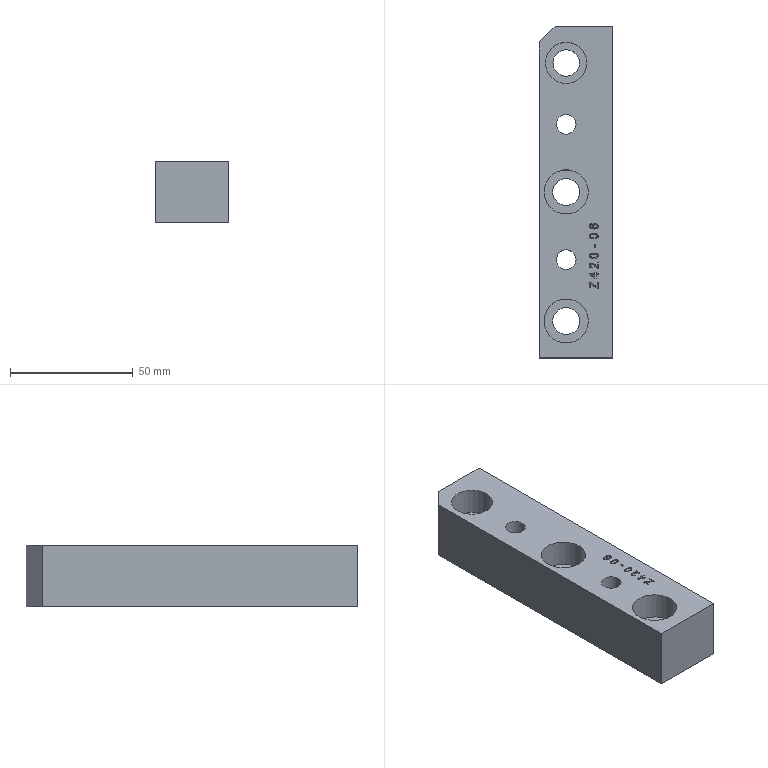Part | Creo | 1 solid | 157 faces | box 30 x 135 x 25 mm | volume 86224 mm3 | other 91 | plane 48 | cylinder 18 | commonest cylinder face diameters 8 x4 11 x4 18 x4 10.8 x2 16.8 x2 3.099 x1